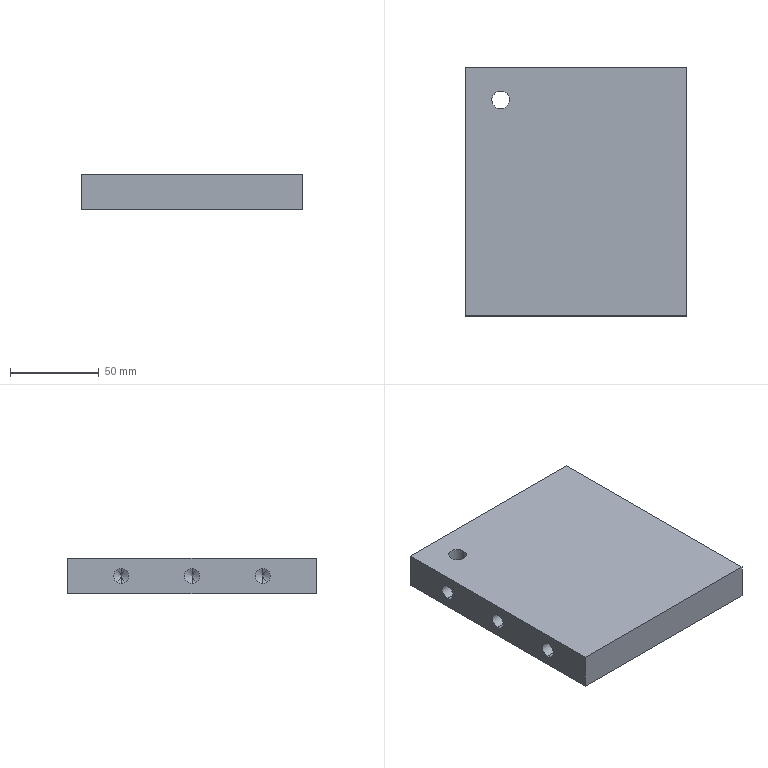Part | SolidWorks | features HoleWzd 2, Extrusion 1, ICE 1 | 1 solid | 32 faces | box 125 x 140 x 20 mm | volume 339828 mm3 | cylinder 14 | cone 12 | plane 6 | commonest cylinder face diameters 6.8 x6 8.5 x6 10 x2
STEP:
#1=CARTESIAN_POINT('',(-47.5,52.,0.));
#2=VERTEX_POINT('',#1);
#3=CARTESIAN_POINT('',(-37.5,52.,0.));
#4=VERTEX_POINT('',#3);
#5=CARTESIAN_POINT('',(-42.5,52.,0.));
#6=DIRECTION('',(0.,0.,1.));
#7=DIRECTION('',(1.,0.,0.));
#8=AXIS2_PLACEMENT_3D('',#5,#6,#7);
#9=CIRCLE('',#8,5.);
#10=EDGE_CURVE('',#2,#4,#9,.T.);
#11=ORIENTED_EDGE('',*,*,#10,.F.);
#12=CARTESIAN_POINT('',(-47.5,52.,20.));
#13=VERTEX_POINT('',#12);
#14=CARTESIAN_POINT('',(-47.5,52.,0.));
#15=DIRECTION('',(0.,0.,1.));
#16=VECTOR('',#15,1000.);
#17=LINE('',#14,#16);
#18=EDGE_CURVE('',#2,#13,#17,.T.);
#19=ORIENTED_EDGE('',*,*,#18,.T.);
#20=CARTESIAN_POINT('',(-37.5,52.,20.));
#21=VERTEX_POINT('',#20);
#22=CARTESIAN_POINT('',(-42.5,52.,20.));
#23=DIRECTION('',(0.,0.,1.));
#24=DIRECTION('',(1.,0.,0.));
#25=AXIS2_PLACEMENT_3D('',#22,#23,#24);
#26=CIRCLE('',#25,5.);
#27=EDGE_CURVE('',#13,#21,#26,.T.);
#28=ORIENTED_EDGE('',*,*,#27,.T.);
#29=CARTESIAN_POINT('',(-37.5,52.,0.));
#30=DIRECTION('',(0.,0.,1.));
#31=VECTOR('',#30,1000.);
#32=LINE('',#29,#31);
#33=EDGE_CURVE('',#4,#21,#32,.T.);
#34=ORIENTED_EDGE('',*,*,#33,.F.);
#35=EDGE_LOOP('',(#11,#19,#28,#34));
#36=FACE_OUTER_BOUND('',#35,.T.);
#37=CARTESIAN_POINT('',(-42.5,52.,0.));
#38=DIRECTION('',(0.,0.,1.));
#39=DIRECTION('',(1.,0.,0.));
#40=AXIS2_PLACEMENT_3D('',#37,#38,#39);
#41=CYLINDRICAL_SURFACE('',#40,5.);
#42=ADVANCED_FACE('',(#36),#41,.F.);
#43=CARTESIAN_POINT('',(40.25,58.,13.4));
#44=VERTEX_POINT('',#43);
#45=CARTESIAN_POINT('',(40.25,58.,6.6));
#46=VERTEX_POINT('',#45);
#47=CARTESIAN_POINT('',(40.25,58.,10.));
#48=DIRECTION('',(1.,0.,0.));
#49=DIRECTION('',(0.,0.,-1.));
#50=AXIS2_PLACEMENT_3D('',#47,#48,#49);
#51=CIRCLE('',#50,3.4);
#52=EDGE_CURVE('',#44,#46,#51,.T.);
#53=ORIENTED_EDGE('',*,*,#52,.F.);
#54=CARTESIAN_POINT('',(62.5,58.,13.4));
#55=VERTEX_POINT('',#54);
#56=CARTESIAN_POINT('',(62.5,58.,13.4));
#57=DIRECTION('',(1.,0.,0.));
#58=VECTOR('',#57,1000.);
#59=LINE('',#56,#58);
#60=EDGE_CURVE('',#44,#55,#59,.T.);
#61=ORIENTED_EDGE('',*,*,#60,.T.);
#62=CARTESIAN_POINT('',(62.5,58.,6.6));
#63=VERTEX_POINT('',#62);
#64=CARTESIAN_POINT('',(62.5,58.,10.));
#65=DIRECTION('',(1.,0.,0.));
#66=DIRECTION('',(0.,0.,-1.));
#67=AXIS2_PLACEMENT_3D('',#64,#65,#66);
#68=CIRCLE('',#67,3.4);
#69=EDGE_CURVE('',#55,#63,#68,.T.);
#70=ORIENTED_EDGE('',*,*,#69,.T.);
#71=CARTESIAN_POINT('',(62.5,58.,6.6));
#72=DIRECTION('',(1.,0.,0.));
#73=VECTOR('',#72,1000.);
#74=LINE('',#71,#73);
#75=EDGE_CURVE('',#46,#63,#74,.T.);
#76=ORIENTED_EDGE('',*,*,#75,.F.);
#77=EDGE_LOOP('',(#53,#61,#70,#76));
#78=FACE_OUTER_BOUND('',#77,.T.);
#79=CARTESIAN_POINT('',(62.5,58.,10.));
#80=DIRECTION('',(1.,0.,0.));
#81=DIRECTION('',(0.,0.,-1.));
#82=AXIS2_PLACEMENT_3D('',#79,#80,#81);
#83=CYLINDRICAL_SURFACE('',#82,3.4);
#84=ADVANCED_FACE('',(#78),#83,.F.);
#85=CARTESIAN_POINT('',(38.207,58.,10.));
#86=VERTEX_POINT('',#85);
#87=CARTESIAN_POINT('',(40.25,58.,6.6));
#88=DIRECTION('',(0.515,0.,-0.8572));
#89=VECTOR('',#88,1000.);
#90=LINE('',#87,#89);
#91=EDGE_CURVE('',#86,#46,#90,.T.);
#92=ORIENTED_EDGE('',*,*,#91,.F.);
#93=CARTESIAN_POINT('',(40.25,58.,13.4));
#94=DIRECTION('',(0.515,0.,0.8572));
#95=VECTOR('',#94,1000.);
#96=LINE('',#93,#95);
#97=EDGE_CURVE('',#86,#44,#96,.T.);
#98=ORIENTED_EDGE('',*,*,#97,.T.);
#99=ORIENTED_EDGE('',*,*,#52,.T.);
#100=EDGE_LOOP('',(#92,#98,#99));
#101=FACE_OUTER_BOUND('',#100,.T.);
#102=CARTESIAN_POINT('',(40.25,58.,10.));
#103=DIRECTION('',(1.,0.,0.));
#104=DIRECTION('',(0.,0.,-1.));
#105=AXIS2_PLACEMENT_3D('',#102,#103,#104);
#106=CONICAL_SURFACE('',#105,3.4,1.03);
#107=ADVANCED_FACE('',(#101),#106,.F.);
#108=CARTESIAN_POINT('',(40.25,0.,13.4));
#109=VERTEX_POINT('',#108);
#110=CARTESIAN_POINT('',(40.25,0.,6.6));
#111=VERTEX_POINT('',#110);
#112=CARTESIAN_POINT('',(40.25,0.,10.));
#113=DIRECTION('',(1.,0.,0.));
#114=DIRECTION('',(0.,0.,-1.));
#115=AXIS2_PLACEMENT_3D('',#112,#113,#114);
#116=CIRCLE('',#115,3.4);
#117=EDGE_CURVE('',#109,#111,#116,.T.);
#118=ORIENTED_EDGE('',*,*,#117,.F.);
#119=CARTESIAN_POINT('',(62.5,0.,13.4));
#120=VERTEX_POINT('',#119);
#121=CARTESIAN_POINT('',(62.5,0.,13.4));
#122=DIRECTION('',(1.,0.,0.));
#123=VECTOR('',#122,1000.);
#124=LINE('',#121,#123);
#125=EDGE_CURVE('',#109,#120,#124,.T.);
#126=ORIENTED_EDGE('',*,*,#125,.T.);
#127=CARTESIAN_POINT('',(62.5,0.,6.6));
#128=VERTEX_POINT('',#127);
#129=CARTESIAN_POINT('',(62.5,0.,10.));
#130=DIRECTION('',(1.,0.,0.));
#131=DIRECTION('',(0.,0.,-1.));
#132=AXIS2_PLACEMENT_3D('',#129,#130,#131);
#133=CIRCLE('',#132,3.4);
#134=EDGE_CURVE('',#120,#128,#133,.T.);
#135=ORIENTED_EDGE('',*,*,#134,.T.);
#136=CARTESIAN_POINT('',(62.5,0.,6.6));
#137=DIRECTION('',(1.,0.,0.));
#138=VECTOR('',#137,1000.);
#139=LINE('',#136,#138);
#140=EDGE_CURVE('',#111,#128,#139,.T.);
#141=ORIENTED_EDGE('',*,*,#140,.F.);
#142=EDGE_LOOP('',(#118,#126,#135,#141));
#143=FACE_OUTER_BOUND('',#142,.T.);
#144=CARTESIAN_POINT('',(62.5,0.,10.));
#145=DIRECTION('',(1.,0.,0.));
#146=DIRECTION('',(0.,0.,-1.));
#147=AXIS2_PLACEMENT_3D('',#144,#145,#146);
#148=CYLINDRICAL_SURFACE('',#147,3.4);
#149=ADVANCED_FACE('',(#143),#148,.F.);
#150=CARTESIAN_POINT('',(38.207,0.,10.));
#151=VERTEX_POINT('',#150);
#152=CARTESIAN_POINT('',(40.25,0.,6.6));
#153=DIRECTION('',(0.515,0.,-0.8572));
#154=VECTOR('',#153,1000.);
#155=LINE('',#152,#154);
#156=EDGE_CURVE('',#151,#111,#155,.T.);
#157=ORIENTED_EDGE('',*,*,#156,.F.);
#158=CARTESIAN_POINT('',(40.25,0.,13.4));
#159=DIRECTION('',(0.515,0.,0.8572));
#160=VECTOR('',#159,1000.);
#161=LINE('',#158,#160);
#162=EDGE_CURVE('',#151,#109,#161,.T.);
#163=ORIENTED_EDGE('',*,*,#162,.T.);
#164=ORIENTED_EDGE('',*,*,#117,.T.);
#165=EDGE_LOOP('',(#157,#163,#164));
#166=FACE_OUTER_BOUND('',#165,.T.);
#167=CARTESIAN_POINT('',(40.25,0.,10.));
#168=DIRECTION('',(1.,0.,0.));
#169=DIRECTION('',(0.,0.,-1.));
#170=AXIS2_PLACEMENT_3D('',#167,#168,#169);
#171=CONICAL_SURFACE('',#170,3.4,1.03);
#172=ADVANCED_FACE('',(#166),#171,.F.);
#173=CARTESIAN_POINT('',(40.25,-58.,13.4));
#174=VERTEX_POINT('',#173);
#175=CARTESIAN_POINT('',(40.25,-58.,6.6));
#176=VERTEX_POINT('',#175);
#177=CARTESIAN_POINT('',(40.25,-58.,10.));
#178=DIRECTION('',(1.,0.,0.));
#179=DIRECTION('',(0.,0.,-1.));
#180=AXIS2_PLACEMENT_3D('',#177,#178,#179);
#181=CIRCLE('',#180,3.4);
#182=EDGE_CURVE('',#174,#176,#181,.T.);
#183=ORIENTED_EDGE('',*,*,#182,.F.);
#184=CARTESIAN_POINT('',(62.5,-58.,13.4));
#185=VERTEX_POINT('',#184);
#186=CARTESIAN_POINT('',(62.5,-58.,13.4));
#187=DIRECTION('',(1.,0.,0.));
#188=VECTOR('',#187,1000.);
#189=LINE('',#186,#188);
#190=EDGE_CURVE('',#174,#185,#189,.T.);
#191=ORIENTED_EDGE('',*,*,#190,.T.);
#192=CARTESIAN_POINT('',(62.5,-58.,6.6));
#193=VERTEX_POINT('',#192);
#194=CARTESIAN_POINT('',(62.5,-58.,10.));
#195=DIRECTION('',(1.,0.,0.));
#196=DIRECTION('',(0.,0.,-1.));
#197=AXIS2_PLACEMENT_3D('',#194,#195,#196);
#198=CIRCLE('',#197,3.4);
#199=EDGE_CURVE('',#185,#193,#198,.T.);
#200=ORIENTED_EDGE('',*,*,#199,.T.);
#201=CARTESIAN_POINT('',(62.5,-58.,6.6));
#202=DIRECTION('',(1.,0.,0.));
#203=VECTOR('',#202,1000.);
#204=LINE('',#201,#203);
#205=EDGE_CURVE('',#176,#193,#204,.T.);
#206=ORIENTED_EDGE('',*,*,#205,.F.);
#207=EDGE_LOOP('',(#183,#191,#200,#206));
#208=FACE_OUTER_BOUND('',#207,.T.);
#209=CARTESIAN_POINT('',(62.5,-58.,10.));
#210=DIRECTION('',(1.,0.,0.));
#211=DIRECTION('',(0.,0.,-1.));
#212=AXIS2_PLACEMENT_3D('',#209,#210,#211);
#213=CYLINDRICAL_SURFACE('',#212,3.4);
#214=ADVANCED_FACE('',(#208),#213,.F.);
#215=CARTESIAN_POINT('',(38.207,-58.,10.));
#216=VERTEX_POINT('',#215);
#217=CARTESIAN_POINT('',(40.25,-58.,6.6));
#218=DIRECTION('',(0.515,0.,-0.8572));
#219=VECTOR('',#218,1000.);
#220=LINE('',#217,#219);
#221=EDGE_CURVE('',#216,#176,#220,.T.);
#222=ORIENTED_EDGE('',*,*,#221,.F.);
#223=CARTESIAN_POINT('',(40.25,-58.,13.4));
#224=DIRECTION('',(0.515,0.,0.8572));
#225=VECTOR('',#224,1000.);
#226=LINE('',#223,#225);
#227=EDGE_CURVE('',#216,#174,#226,.T.);
#228=ORIENTED_EDGE('',*,*,#227,.T.);
#229=ORIENTED_EDGE('',*,*,#182,.T.);
#230=EDGE_LOOP('',(#222,#228,#229));
#231=FACE_OUTER_BOUND('',#230,.T.);
#232=CARTESIAN_POINT('',(40.25,-58.,10.));
#233=DIRECTION('',(1.,0.,0.));
#234=DIRECTION('',(0.,0.,-1.));
#235=AXIS2_PLACEMENT_3D('',#232,#233,#234);
#236=CONICAL_SURFACE('',#235,3.4,1.03);
#237=ADVANCED_FACE('',(#231),#236,.F.);
#238=CARTESIAN_POINT('',(-27.5,40.,5.75));
#239=VERTEX_POINT('',#238);
#240=CARTESIAN_POINT('',(-27.5,40.,14.25));
#241=VERTEX_POINT('',#240);
#242=CARTESIAN_POINT('',(-27.5,40.,10.));
#243=DIRECTION('',(-1.,0.,0.));
#244=DIRECTION('',(0.,0.,1.));
#245=AXIS2_PLACEMENT_3D('',#242,#243,#244);
#246=CIRCLE('',#245,4.25);
#247=EDGE_CURVE('',#239,#241,#246,.T.);
#248=ORIENTED_EDGE('',*,*,#247,.F.);
#249=CARTESIAN_POINT('',(-62.5,40.,5.75));
#250=VERTEX_POINT('',#249);
#251=CARTESIAN_POINT('',(-62.5,40.,5.75));
#252=DIRECTION('',(-1.,0.,0.));
#253=VECTOR('',#252,1000.);
#254=LINE('',#251,#253);
#255=EDGE_CURVE('',#239,#250,#254,.T.);
#256=ORIENTED_EDGE('',*,*,#255,.T.);
#257=CARTESIAN_POINT('',(-62.5,40.,14.25));
#258=VERTEX_POINT('',#257);
#259=CARTESIAN_POINT('',(-62.5,40.,10.));
#260=DIRECTION('',(-1.,0.,0.));
#261=DIRECTION('',(0.,0.,1.));
#262=AXIS2_PLACEMENT_3D('',#259,#260,#261);
#263=CIRCLE('',#262,4.25);
#264=EDGE_CURVE('',#250,#258,#263,.T.);
#265=ORIENTED_EDGE('',*,*,#264,.T.);
#266=CARTESIAN_POINT('',(-62.5,40.,14.25));
#267=DIRECTION('',(-1.,0.,0.));
#268=VECTOR('',#267,1000.);
#269=LINE('',#266,#268);
#270=EDGE_CURVE('',#241,#258,#269,.T.);
#271=ORIENTED_EDGE('',*,*,#270,.F.);
#272=EDGE_LOOP('',(#248,#256,#265,#271));
#273=FACE_OUTER_BOUND('',#272,.T.);
#274=CARTESIAN_POINT('',(-62.5,40.,10.));
#275=DIRECTION('',(-1.,0.,0.));
#276=DIRECTION('',(0.,0.,1.));
#277=AXIS2_PLACEMENT_3D('',#274,#275,#276);
#278=CYLINDRICAL_SURFACE('',#277,4.25);
#279=ADVANCED_FACE('',(#273),#278,.F.);
#280=CARTESIAN_POINT('',(-24.946,40.,10.));
#281=VERTEX_POINT('',#280);
#282=CARTESIAN_POINT('',(-27.5,40.,14.25));
#283=DIRECTION('',(-0.515,0.,0.8572));
#284=VECTOR('',#283,1000.);
#285=LINE('',#282,#284);
#286=EDGE_CURVE('',#281,#241,#285,.T.);
#287=ORIENTED_EDGE('',*,*,#286,.F.);
#288=CARTESIAN_POINT('',(-27.5,40.,5.75));
#289=DIRECTION('',(-0.515,0.,-0.8572));
#290=VECTOR('',#289,1000.);
#291=LINE('',#288,#290);
#292=EDGE_CURVE('',#281,#239,#291,.T.);
#293=ORIENTED_EDGE('',*,*,#292,.T.);
#294=ORIENTED_EDGE('',*,*,#247,.T.);
#295=EDGE_LOOP('',(#287,#293,#294));
#296=FACE_OUTER_BOUND('',#295,.T.);
#297=CARTESIAN_POINT('',(-27.5,40.,10.));
#298=DIRECTION('',(-1.,0.,0.));
#299=DIRECTION('',(0.,0.,1.));
#300=AXIS2_PLACEMENT_3D('',#297,#298,#299);
#301=CONICAL_SURFACE('',#300,4.25,1.03);
#302=ADVANCED_FACE('',(#296),#301,.F.);
#303=CARTESIAN_POINT('',(-27.5,0.,5.75));
#304=VERTEX_POINT('',#303);
#305=CARTESIAN_POINT('',(-27.5,0.,14.25));
#306=VERTEX_POINT('',#305);
#307=CARTESIAN_POINT('',(-27.5,0.,10.));
#308=DIRECTION('',(-1.,0.,0.));
#309=DIRECTION('',(0.,0.,1.));
#310=AXIS2_PLACEMENT_3D('',#307,#308,#309);
#311=CIRCLE('',#310,4.25);
#312=EDGE_CURVE('',#304,#306,#311,.T.);
#313=ORIENTED_EDGE('',*,*,#312,.F.);
#314=CARTESIAN_POINT('',(-62.5,0.,5.75));
#315=VERTEX_POINT('',#314);
#316=CARTESIAN_POINT('',(-62.5,0.,5.75));
#317=DIRECTION('',(-1.,0.,0.));
#318=VECTOR('',#317,1000.);
#319=LINE('',#316,#318);
#320=EDGE_CURVE('',#304,#315,#319,.T.);
#321=ORIENTED_EDGE('',*,*,#320,.T.);
#322=CARTESIAN_POINT('',(-62.5,0.,14.25));
#323=VERTEX_POINT('',#322);
#324=CARTESIAN_POINT('',(-62.5,0.,10.));
#325=DIRECTION('',(-1.,0.,0.));
#326=DIRECTION('',(0.,0.,1.));
#327=AXIS2_PLACEMENT_3D('',#324,#325,#326);
#328=CIRCLE('',#327,4.25);
#329=EDGE_CURVE('',#315,#323,#328,.T.);
#330=ORIENTED_EDGE('',*,*,#329,.T.);
#331=CARTESIAN_POINT('',(-62.5,0.,14.25));
#332=DIRECTION('',(-1.,0.,0.));
#333=VECTOR('',#332,1000.);
#334=LINE('',#331,#333);
#335=EDGE_CURVE('',#306,#323,#334,.T.);
#336=ORIENTED_EDGE('',*,*,#335,.F.);
#337=EDGE_LOOP('',(#313,#321,#330,#336));
#338=FACE_OUTER_BOUND('',#337,.T.);
#339=CARTESIAN_POINT('',(-62.5,0.,10.));
#340=DIRECTION('',(-1.,0.,0.));
#341=DIRECTION('',(0.,0.,1.));
#342=AXIS2_PLACEMENT_3D('',#339,#340,#341);
#343=CYLINDRICAL_SURFACE('',#342,4.25);
#344=ADVANCED_FACE('',(#338),#343,.F.);
#345=CARTESIAN_POINT('',(-24.946,0.,10.));
#346=VERTEX_POINT('',#345);
#347=CARTESIAN_POINT('',(-27.5,0.,14.25));
#348=DIRECTION('',(-0.515,0.,0.8572));
#349=VECTOR('',#348,1000.);
#350=LINE('',#347,#349);
#351=EDGE_CURVE('',#346,#306,#350,.T.);
#352=ORIENTED_EDGE('',*,*,#351,.F.);
#353=CARTESIAN_POINT('',(-27.5,0.,5.75));
#354=DIRECTION('',(-0.515,0.,-0.8572));
#355=VECTOR('',#354,1000.);
#356=LINE('',#353,#355);
#357=EDGE_CURVE('',#346,#304,#356,.T.);
#358=ORIENTED_EDGE('',*,*,#357,.T.);
#359=ORIENTED_EDGE('',*,*,#312,.T.);
#360=EDGE_LOOP('',(#352,#358,#359));
#361=FACE_OUTER_BOUND('',#360,.T.);
#362=CARTESIAN_POINT('',(-27.5,0.,10.));
#363=DIRECTION('',(-1.,0.,0.));
#364=DIRECTION('',(0.,0.,1.));
#365=AXIS2_PLACEMENT_3D('',#362,#363,#364);
#366=CONICAL_SURFACE('',#365,4.25,1.03);
#367=ADVANCED_FACE('',(#361),#366,.F.);
#368=CARTESIAN_POINT('',(-27.5,-40.,5.75));
#369=VERTEX_POINT('',#368);
#370=CARTESIAN_POINT('',(-27.5,-40.,14.25));
#371=VERTEX_POINT('',#370);
#372=CARTESIAN_POINT('',(-27.5,-40.,10.));
#373=DIRECTION('',(-1.,0.,0.));
#374=DIRECTION('',(0.,0.,1.));
#375=AXIS2_PLACEMENT_3D('',#372,#373,#374);
#376=CIRCLE('',#375,4.25);
#377=EDGE_CURVE('',#369,#371,#376,.T.);
#378=ORIENTED_EDGE('',*,*,#377,.F.);
#379=CARTESIAN_POINT('',(-62.5,-40.,5.75));
#380=VERTEX_POINT('',#379);
#381=CARTESIAN_POINT('',(-62.5,-40.,5.75));
#382=DIRECTION('',(-1.,0.,0.));
#383=VECTOR('',#382,1000.);
#384=LINE('',#381,#383);
#385=EDGE_CURVE('',#369,#380,#384,.T.);
#386=ORIENTED_EDGE('',*,*,#385,.T.);
#387=CARTESIAN_POINT('',(-62.5,-40.,14.25));
#388=VERTEX_POINT('',#387);
#389=CARTESIAN_POINT('',(-62.5,-40.,10.));
#390=DIRECTION('',(-1.,0.,0.));
#391=DIRECTION('',(0.,0.,1.));
#392=AXIS2_PLACEMENT_3D('',#389,#390,#391);
#393=CIRCLE('',#392,4.25);
#394=EDGE_CURVE('',#380,#388,#393,.T.);
#395=ORIENTED_EDGE('',*,*,#394,.T.);
#396=CARTESIAN_POINT('',(-62.5,-40.,14.25));
#397=DIRECTION('',(-1.,0.,0.));
#398=VECTOR('',#397,1000.);
#399=LINE('',#396,#398);
#400=EDGE_CURVE('',#371,#388,#399,.T.);
#401=ORIENTED_EDGE('',*,*,#400,.F.);
#402=EDGE_LOOP('',(#378,#386,#395,#401));
#403=FACE_OUTER_BOUND('',#402,.T.);
#404=CARTESIAN_POINT('',(-62.5,-40.,10.));
#405=DIRECTION('',(-1.,0.,0.));
#406=DIRECTION('',(0.,0.,1.));
#407=AXIS2_PLACEMENT_3D('',#404,#405,#406);
#408=CYLINDRICAL_SURFACE('',#407,4.25);
#409=ADVANCED_FACE('',(#403),#408,.F.);
#410=CARTESIAN_POINT('',(-24.946,-40.,10.));
#411=VERTEX_POINT('',#410);
#412=CARTESIAN_POINT('',(-27.5,-40.,14.25));
#413=DIRECTION('',(-0.515,0.,0.8572));
#414=VECTOR('',#413,1000.);
#415=LINE('',#412,#414);
#416=EDGE_CURVE('',#411,#371,#415,.T.);
#417=ORIENTED_EDGE('',*,*,#416,.F.);
#418=CARTESIAN_POINT('',(-27.5,-40.,5.75));
#419=DIRECTION('',(-0.515,0.,-0.8572));
#420=VECTOR('',#419,1000.);
#421=LINE('',#418,#420);
#422=EDGE_CURVE('',#411,#369,#421,.T.);
#423=ORIENTED_EDGE('',*,*,#422,.T.);
#424=ORIENTED_EDGE('',*,*,#377,.T.);
#425=EDGE_LOOP('',(#417,#423,#424));
#426=FACE_OUTER_BOUND('',#425,.T.);
#427=CARTESIAN_POINT('',(-27.5,-40.,10.));
#428=DIRECTION('',(-1.,0.,0.));
#429=DIRECTION('',(0.,0.,1.));
#430=AXIS2_PLACEMENT_3D('',#427,#428,#429);
#431=CONICAL_SURFACE('',#430,4.25,1.03);
#432=ADVANCED_FACE('',(#426),#431,.F.);
#433=CARTESIAN_POINT('',(62.5,58.,10.));
#434=DIRECTION('',(1.,0.,0.));
#435=DIRECTION('',(0.,0.,-1.));
#436=AXIS2_PLACEMENT_3D('',#433,#434,#435);
#437=CIRCLE('',#436,3.4);
#438=EDGE_CURVE('',#63,#55,#437,.T.);
#439=ORIENTED_EDGE('',*,*,#438,.F.);
#440=ORIENTED_EDGE('',*,*,#69,.F.);
#441=EDGE_LOOP('',(#439,#440));
#442=FACE_BOUND('',#441,.T.);
#443=CARTESIAN_POINT('',(62.5,0.,10.));
#444=DIRECTION('',(1.,0.,0.));
#445=DIRECTION('',(0.,0.,-1.));
#446=AXIS2_PLACEMENT_3D('',#443,#444,#445);
#447=CIRCLE('',#446,3.4);
#448=EDGE_CURVE('',#128,#120,#447,.T.);
#449=ORIENTED_EDGE('',*,*,#448,.F.);
#450=ORIENTED_EDGE('',*,*,#134,.F.);
#451=EDGE_LOOP('',(#449,#450));
#452=FACE_BOUND('',#451,.T.);
#453=CARTESIAN_POINT('',(62.5,-58.,10.));
#454=DIRECTION('',(1.,0.,0.));
#455=DIRECTION('',(0.,0.,-1.));
#456=AXIS2_PLACEMENT_3D('',#453,#454,#455);
#457=CIRCLE('',#456,3.4);
#458=EDGE_CURVE('',#193,#185,#457,.T.);
#459=ORIENTED_EDGE('',*,*,#458,.F.);
#460=ORIENTED_EDGE('',*,*,#199,.F.);
#461=EDGE_LOOP('',(#459,#460));
#462=FACE_BOUND('',#461,.T.);
#463=CARTESIAN_POINT('',(62.5,-70.,0.));
#464=VERTEX_POINT('',#463);
#465=CARTESIAN_POINT('',(62.5,70.,0.));
#466=VERTEX_POINT('',#465);
#467=CARTESIAN_POINT('',(62.5,70.,0.));
#468=DIRECTION('',(0.,1.,0.));
#469=VECTOR('',#468,1000.);
#470=LINE('',#467,#469);
#471=EDGE_CURVE('',#464,#466,#470,.T.);
#472=ORIENTED_EDGE('',*,*,#471,.T.);
#473=CARTESIAN_POINT('',(62.5,70.,20.));
#474=VERTEX_POINT('',#473);
#475=CARTESIAN_POINT('',(62.5,70.,20.));
#476=DIRECTION('',(0.,0.,-1.));
#477=VECTOR('',#476,1000.);
#478=LINE('',#475,#477);
#479=EDGE_CURVE('',#474,#466,#478,.T.);
#480=ORIENTED_EDGE('',*,*,#479,.F.);
#481=CARTESIAN_POINT('',(62.5,-70.,20.));
#482=VERTEX_POINT('',#481);
#483=CARTESIAN_POINT('',(62.5,70.,20.));
#484=DIRECTION('',(0.,1.,0.));
#485=VECTOR('',#484,1000.);
#486=LINE('',#483,#485);
#487=EDGE_CURVE('',#482,#474,#486,.T.);
#488=ORIENTED_EDGE('',*,*,#487,.F.);
#489=CARTESIAN_POINT('',(62.5,-70.,20.));
#490=DIRECTION('',(0.,0.,-1.));
#491=VECTOR('',#490,1000.);
#492=LINE('',#489,#491);
#493=EDGE_CURVE('',#482,#464,#492,.T.);
#494=ORIENTED_EDGE('',*,*,#493,.T.);
#495=EDGE_LOOP('',(#472,#480,#488,#494));
#496=FACE_OUTER_BOUND('',#495,.T.);
#497=CARTESIAN_POINT('',(62.5,70.,20.));
#498=DIRECTION('',(-1.,0.,0.));
#499=DIRECTION('',(0.,-1.,0.));
#500=AXIS2_PLACEMENT_3D('',#497,#498,#499);
#501=PLANE('',#500);
#502=ADVANCED_FACE('',(#442,#452,#462,#496),#501,.F.);
#503=CARTESIAN_POINT('',(-62.5,70.,0.));
#504=VERTEX_POINT('',#503);
#505=CARTESIAN_POINT('',(-62.5,70.,0.));
#506=DIRECTION('',(-1.,0.,0.));
#507=VECTOR('',#506,1000.);
#508=LINE('',#505,#507);
#509=EDGE_CURVE('',#466,#504,#508,.T.);
#510=ORIENTED_EDGE('',*,*,#509,.T.);
#511=CARTESIAN_POINT('',(-62.5,70.,20.));
#512=VERTEX_POINT('',#511);
#513=CARTESIAN_POINT('',(-62.5,70.,20.));
#514=DIRECTION('',(0.,0.,-1.));
#515=VECTOR('',#514,1000.);
#516=LINE('',#513,#515);
#517=EDGE_CURVE('',#512,#504,#516,.T.);
#518=ORIENTED_EDGE('',*,*,#517,.F.);
#519=CARTESIAN_POINT('',(-62.5,70.,20.));
#520=DIRECTION('',(-1.,0.,0.));
#521=VECTOR('',#520,1000.);
#522=LINE('',#519,#521);
#523=EDGE_CURVE('',#474,#512,#522,.T.);
#524=ORIENTED_EDGE('',*,*,#523,.F.);
#525=ORIENTED_EDGE('',*,*,#479,.T.);
#526=EDGE_LOOP('',(#510,#518,#524,#525));
#527=FACE_OUTER_BOUND('',#526,.T.);
#528=CARTESIAN_POINT('',(-62.5,70.,20.));
#529=DIRECTION('',(0.,-1.,0.));
#530=DIRECTION('',(0.,0.,-1.));
#531=AXIS2_PLACEMENT_3D('',#528,#529,#530);
#532=PLANE('',#531);
#533=ADVANCED_FACE('',(#527),#532,.F.);
#534=CARTESIAN_POINT('',(-62.5,40.,10.));
#535=DIRECTION('',(-1.,0.,0.));
#536=DIRECTION('',(0.,0.,1.));
#537=AXIS2_PLACEMENT_3D('',#534,#535,#536);
#538=CIRCLE('',#537,4.25);
#539=EDGE_CURVE('',#258,#250,#538,.T.);
#540=ORIENTED_EDGE('',*,*,#539,.F.);
#541=ORIENTED_EDGE('',*,*,#264,.F.);
#542=EDGE_LOOP('',(#540,#541));
#543=FACE_BOUND('',#542,.T.);
#544=CARTESIAN_POINT('',(-62.5,0.,10.));
#545=DIRECTION('',(-1.,0.,0.));
#546=DIRECTION('',(0.,0.,1.));
#547=AXIS2_PLACEMENT_3D('',#544,#545,#546);
#548=CIRCLE('',#547,4.25);
#549=EDGE_CURVE('',#323,#315,#548,.T.);
#550=ORIENTED_EDGE('',*,*,#549,.F.);
#551=ORIENTED_EDGE('',*,*,#329,.F.);
#552=EDGE_LOOP('',(#550,#551));
#553=FACE_BOUND('',#552,.T.);
#554=CARTESIAN_POINT('',(-62.5,-40.,10.));
#555=DIRECTION('',(-1.,0.,0.));
#556=DIRECTION('',(0.,0.,1.));
#557=AXIS2_PLACEMENT_3D('',#554,#555,#556);
#558=CIRCLE('',#557,4.25);
#559=EDGE_CURVE('',#388,#380,#558,.T.);
#560=ORIENTED_EDGE('',*,*,#559,.F.);
#561=ORIENTED_EDGE('',*,*,#394,.F.);
#562=EDGE_LOOP('',(#560,#561));
#563=FACE_BOUND('',#562,.T.);
#564=CARTESIAN_POINT('',(-62.5,-70.,0.));
#565=VERTEX_POINT('',#564);
#566=CARTESIAN_POINT('',(-62.5,70.,0.));
#567=DIRECTION('',(0.,-1.,0.));
#568=VECTOR('',#567,1000.);
#569=LINE('',#566,#568);
#570=EDGE_CURVE('',#504,#565,#569,.T.);
#571=ORIENTED_EDGE('',*,*,#570,.T.);
#572=CARTESIAN_POINT('',(-62.5,-70.,20.));
#573=VERTEX_POINT('',#572);
#574=CARTESIAN_POINT('',(-62.5,-70.,20.));
#575=DIRECTION('',(0.,0.,-1.));
#576=VECTOR('',#575,1000.);
#577=LINE('',#574,#576);
#578=EDGE_CURVE('',#573,#565,#577,.T.);
#579=ORIENTED_EDGE('',*,*,#578,.F.);
#580=CARTESIAN_POINT('',(-62.5,70.,20.));
#581=DIRECTION('',(0.,-1.,0.));
#582=VECTOR('',#581,1000.);
#583=LINE('',#580,#582);
#584=EDGE_CURVE('',#512,#573,#583,.T.);
#585=ORIENTED_EDGE('',*,*,#584,.F.);
#586=ORIENTED_EDGE('',*,*,#517,.T.);
#587=EDGE_LOOP('',(#571,#579,#585,#586));
#588=FACE_OUTER_BOUND('',#587,.T.);
#589=CARTESIAN_POINT('',(-62.5,70.,20.));
#590=DIRECTION('',(1.,0.,0.));
#591=DIRECTION('',(0.,1.,0.));
#592=AXIS2_PLACEMENT_3D('',#589,#590,#591);
#593=PLANE('',#592);
#594=ADVANCED_FACE('',(#543,#553,#563,#588),#593,.F.);
#595=CARTESIAN_POINT('',(-62.5,-70.,0.));
#596=DIRECTION('',(1.,0.,0.));
#597=VECTOR('',#596,1000.);
#598=LINE('',#595,#597);
#599=EDGE_CURVE('',#565,#464,#598,.T.);
#600=ORIENTED_EDGE('',*,*,#599,.T.);
#601=ORIENTED_EDGE('',*,*,#493,.F.);
#602=CARTESIAN_POINT('',(-62.5,-70.,20.));
#603=DIRECTION('',(1.,0.,0.));
#604=VECTOR('',#603,1000.);
#605=LINE('',#602,#604);
#606=EDGE_CURVE('',#573,#482,#605,.T.);
#607=ORIENTED_EDGE('',*,*,#606,.F.);
#608=ORIENTED_EDGE('',*,*,#578,.T.);
#609=EDGE_LOOP('',(#600,#601,#607,#608));
#610=FACE_OUTER_BOUND('',#609,.T.);
#611=CARTESIAN_POINT('',(-62.5,-70.,20.));
#612=DIRECTION('',(0.,1.,0.));
#613=DIRECTION('',(0.,0.,1.));
#614=AXIS2_PLACEMENT_3D('',#611,#612,#613);
#615=PLANE('',#614);
#616=ADVANCED_FACE('',(#610),#615,.F.);
#617=CARTESIAN_POINT('',(-42.5,52.,20.));
#618=DIRECTION('',(0.,0.,1.));
#619=DIRECTION('',(1.,0.,0.));
#620=AXIS2_PLACEMENT_3D('',#617,#618,#619);
#621=CIRCLE('',#620,5.);
#622=EDGE_CURVE('',#21,#13,#621,.T.);
#623=ORIENTED_EDGE('',*,*,#622,.F.);
#624=ORIENTED_EDGE('',*,*,#27,.F.);
#625=EDGE_LOOP('',(#623,#624));
#626=FACE_BOUND('',#625,.T.);
#627=ORIENTED_EDGE('',*,*,#487,.T.);
#628=ORIENTED_EDGE('',*,*,#523,.T.);
#629=ORIENTED_EDGE('',*,*,#584,.T.);
#630=ORIENTED_EDGE('',*,*,#606,.T.);
#631=EDGE_LOOP('',(#627,#628,#629,#630));
#632=FACE_OUTER_BOUND('',#631,.T.);
#633=CARTESIAN_POINT('',(0.,0.,20.));
#634=DIRECTION('',(0.,0.,1.));
#635=DIRECTION('',(1.,0.,0.));
#636=AXIS2_PLACEMENT_3D('',#633,#634,#635);
#637=PLANE('',#636);
#638=ADVANCED_FACE('',(#626,#632),#637,.T.);
#639=CARTESIAN_POINT('',(-42.5,52.,0.));
#640=DIRECTION('',(0.,0.,1.));
#641=DIRECTION('',(1.,0.,0.));
#642=AXIS2_PLACEMENT_3D('',#639,#640,#641);
#643=CIRCLE('',#642,5.);
#644=EDGE_CURVE('',#4,#2,#643,.T.);
#645=ORIENTED_EDGE('',*,*,#644,.T.);
#646=ORIENTED_EDGE('',*,*,#10,.T.);
#647=EDGE_LOOP('',(#645,#646));
#648=FACE_BOUND('',#647,.T.);
#649=ORIENTED_EDGE('',*,*,#471,.F.);
#650=ORIENTED_EDGE('',*,*,#599,.F.);
#651=ORIENTED_EDGE('',*,*,#570,.F.);
#652=ORIENTED_EDGE('',*,*,#509,.F.);
#653=EDGE_LOOP('',(#649,#650,#651,#652));
#654=FACE_OUTER_BOUND('',#653,.T.);
#655=CARTESIAN_POINT('',(0.,0.,0.));
#656=DIRECTION('',(0.,0.,1.));
#657=DIRECTION('',(1.,0.,0.));
#658=AXIS2_PLACEMENT_3D('',#655,#656,#657);
#659=PLANE('',#658);
#660=ADVANCED_FACE('',(#648,#654),#659,.F.);
#661=ORIENTED_EDGE('',*,*,#422,.F.);
#662=ORIENTED_EDGE('',*,*,#416,.T.);
#663=CARTESIAN_POINT('',(-27.5,-40.,10.));
#664=DIRECTION('',(-1.,0.,0.));
#665=DIRECTION('',(0.,0.,1.));
#666=AXIS2_PLACEMENT_3D('',#663,#664,#665);
#667=CIRCLE('',#666,4.25);
#668=EDGE_CURVE('',#371,#369,#667,.T.);
#669=ORIENTED_EDGE('',*,*,#668,.T.);
#670=EDGE_LOOP('',(#661,#662,#669));
#671=FACE_OUTER_BOUND('',#670,.T.);
#672=CARTESIAN_POINT('',(-27.5,-40.,10.));
#673=DIRECTION('',(-1.,0.,0.));
#674=DIRECTION('',(0.,0.,1.));
#675=AXIS2_PLACEMENT_3D('',#672,#673,#674);
#676=CONICAL_SURFACE('',#675,4.25,1.03);
#677=ADVANCED_FACE('',(#671),#676,.F.);
#678=ORIENTED_EDGE('',*,*,#385,.F.);
#679=ORIENTED_EDGE('',*,*,#668,.F.);
#680=ORIENTED_EDGE('',*,*,#400,.T.);
#681=ORIENTED_EDGE('',*,*,#559,.T.);
#682=EDGE_LOOP('',(#678,#679,#680,#681));
#683=FACE_OUTER_BOUND('',#682,.T.);
#684=CARTESIAN_POINT('',(-62.5,-40.,10.));
#685=DIRECTION('',(-1.,0.,0.));
#686=DIRECTION('',(0.,0.,1.));
#687=AXIS2_PLACEMENT_3D('',#684,#685,#686);
#688=CYLINDRICAL_SURFACE('',#687,4.25);
#689=ADVANCED_FACE('',(#683),#688,.F.);
#690=ORIENTED_EDGE('',*,*,#357,.F.);
#691=ORIENTED_EDGE('',*,*,#351,.T.);
#692=CARTESIAN_POINT('',(-27.5,0.,10.));
#693=DIRECTION('',(-1.,0.,0.));
#694=DIRECTION('',(0.,0.,1.));
#695=AXIS2_PLACEMENT_3D('',#692,#693,#694);
#696=CIRCLE('',#695,4.25);
#697=EDGE_CURVE('',#306,#304,#696,.T.);
#698=ORIENTED_EDGE('',*,*,#697,.T.);
#699=EDGE_LOOP('',(#690,#691,#698));
#700=FACE_OUTER_BOUND('',#699,.T.);
#701=CARTESIAN_POINT('',(-27.5,0.,10.));
#702=DIRECTION('',(-1.,0.,0.));
#703=DIRECTION('',(0.,0.,1.));
#704=AXIS2_PLACEMENT_3D('',#701,#702,#703);
#705=CONICAL_SURFACE('',#704,4.25,1.03);
#706=ADVANCED_FACE('',(#700),#705,.F.);
#707=ORIENTED_EDGE('',*,*,#320,.F.);
#708=ORIENTED_EDGE('',*,*,#697,.F.);
#709=ORIENTED_EDGE('',*,*,#335,.T.);
#710=ORIENTED_EDGE('',*,*,#549,.T.);
#711=EDGE_LOOP('',(#707,#708,#709,#710));
#712=FACE_OUTER_BOUND('',#711,.T.);
#713=CARTESIAN_POINT('',(-62.5,0.,10.));
#714=DIRECTION('',(-1.,0.,0.));
#715=DIRECTION('',(0.,0.,1.));
#716=AXIS2_PLACEMENT_3D('',#713,#714,#715);
#717=CYLINDRICAL_SURFACE('',#716,4.25);
#718=ADVANCED_FACE('',(#712),#717,.F.);
#719=ORIENTED_EDGE('',*,*,#292,.F.);
#720=ORIENTED_EDGE('',*,*,#286,.T.);
#721=CARTESIAN_POINT('',(-27.5,40.,10.));
#722=DIRECTION('',(-1.,0.,0.));
#723=DIRECTION('',(0.,0.,1.));
#724=AXIS2_PLACEMENT_3D('',#721,#722,#723);
#725=CIRCLE('',#724,4.25);
#726=EDGE_CURVE('',#241,#239,#725,.T.);
#727=ORIENTED_EDGE('',*,*,#726,.T.);
#728=EDGE_LOOP('',(#719,#720,#727));
#729=FACE_OUTER_BOUND('',#728,.T.);
#730=CARTESIAN_POINT('',(-27.5,40.,10.));
#731=DIRECTION('',(-1.,0.,0.));
#732=DIRECTION('',(0.,0.,1.));
#733=AXIS2_PLACEMENT_3D('',#730,#731,#732);
#734=CONICAL_SURFACE('',#733,4.25,1.03);
#735=ADVANCED_FACE('',(#729),#734,.F.);
#736=ORIENTED_EDGE('',*,*,#255,.F.);
#737=ORIENTED_EDGE('',*,*,#726,.F.);
#738=ORIENTED_EDGE('',*,*,#270,.T.);
#739=ORIENTED_EDGE('',*,*,#539,.T.);
#740=EDGE_LOOP('',(#736,#737,#738,#739));
#741=FACE_OUTER_BOUND('',#740,.T.);
#742=CARTESIAN_POINT('',(-62.5,40.,10.));
#743=DIRECTION('',(-1.,0.,0.));
#744=DIRECTION('',(0.,0.,1.));
#745=AXIS2_PLACEMENT_3D('',#742,#743,#744);
#746=CYLINDRICAL_SURFACE('',#745,4.25);
#747=ADVANCED_FACE('',(#741),#746,.F.);
#748=ORIENTED_EDGE('',*,*,#227,.F.);
#749=ORIENTED_EDGE('',*,*,#221,.T.);
#750=CARTESIAN_POINT('',(40.25,-58.,10.));
#751=DIRECTION('',(1.,0.,0.));
#752=DIRECTION('',(0.,0.,-1.));
#753=AXIS2_PLACEMENT_3D('',#750,#751,#752);
#754=CIRCLE('',#753,3.4);
#755=EDGE_CURVE('',#176,#174,#754,.T.);
#756=ORIENTED_EDGE('',*,*,#755,.T.);
#757=EDGE_LOOP('',(#748,#749,#756));
#758=FACE_OUTER_BOUND('',#757,.T.);
#759=CARTESIAN_POINT('',(40.25,-58.,10.));
#760=DIRECTION('',(1.,0.,0.));
#761=DIRECTION('',(0.,0.,-1.));
#762=AXIS2_PLACEMENT_3D('',#759,#760,#761);
#763=CONICAL_SURFACE('',#762,3.4,1.03);
#764=ADVANCED_FACE('',(#758),#763,.F.);
#765=ORIENTED_EDGE('',*,*,#190,.F.);
#766=ORIENTED_EDGE('',*,*,#755,.F.);
#767=ORIENTED_EDGE('',*,*,#205,.T.);
#768=ORIENTED_EDGE('',*,*,#458,.T.);
#769=EDGE_LOOP('',(#765,#766,#767,#768));
#770=FACE_OUTER_BOUND('',#769,.T.);
#771=CARTESIAN_POINT('',(62.5,-58.,10.));
#772=DIRECTION('',(1.,0.,0.));
#773=DIRECTION('',(0.,0.,-1.));
#774=AXIS2_PLACEMENT_3D('',#771,#772,#773);
#775=CYLINDRICAL_SURFACE('',#774,3.4);
#776=ADVANCED_FACE('',(#770),#775,.F.);
#777=ORIENTED_EDGE('',*,*,#162,.F.);
#778=ORIENTED_EDGE('',*,*,#156,.T.);
#779=CARTESIAN_POINT('',(40.25,0.,10.));
#780=DIRECTION('',(1.,0.,0.));
#781=DIRECTION('',(0.,0.,-1.));
#782=AXIS2_PLACEMENT_3D('',#779,#780,#781);
#783=CIRCLE('',#782,3.4);
#784=EDGE_CURVE('',#111,#109,#783,.T.);
#785=ORIENTED_EDGE('',*,*,#784,.T.);
#786=EDGE_LOOP('',(#777,#778,#785));
#787=FACE_OUTER_BOUND('',#786,.T.);
#788=CARTESIAN_POINT('',(40.25,0.,10.));
#789=DIRECTION('',(1.,0.,0.));
#790=DIRECTION('',(0.,0.,-1.));
#791=AXIS2_PLACEMENT_3D('',#788,#789,#790);
#792=CONICAL_SURFACE('',#791,3.4,1.03);
#793=ADVANCED_FACE('',(#787),#792,.F.);
#794=ORIENTED_EDGE('',*,*,#125,.F.);
#795=ORIENTED_EDGE('',*,*,#784,.F.);
#796=ORIENTED_EDGE('',*,*,#140,.T.);
#797=ORIENTED_EDGE('',*,*,#448,.T.);
#798=EDGE_LOOP('',(#794,#795,#796,#797));
#799=FACE_OUTER_BOUND('',#798,.T.);
#800=CARTESIAN_POINT('',(62.5,0.,10.));
#801=DIRECTION('',(1.,0.,0.));
#802=DIRECTION('',(0.,0.,-1.));
#803=AXIS2_PLACEMENT_3D('',#800,#801,#802);
#804=CYLINDRICAL_SURFACE('',#803,3.4);
#805=ADVANCED_FACE('',(#799),#804,.F.);
#806=ORIENTED_EDGE('',*,*,#97,.F.);
#807=ORIENTED_EDGE('',*,*,#91,.T.);
#808=CARTESIAN_POINT('',(40.25,58.,10.));
#809=DIRECTION('',(1.,0.,0.));
#810=DIRECTION('',(0.,0.,-1.));
#811=AXIS2_PLACEMENT_3D('',#808,#809,#810);
#812=CIRCLE('',#811,3.4);
#813=EDGE_CURVE('',#46,#44,#812,.T.);
#814=ORIENTED_EDGE('',*,*,#813,.T.);
#815=EDGE_LOOP('',(#806,#807,#814));
#816=FACE_OUTER_BOUND('',#815,.T.);
#817=CARTESIAN_POINT('',(40.25,58.,10.));
#818=DIRECTION('',(1.,0.,0.));
#819=DIRECTION('',(0.,0.,-1.));
#820=AXIS2_PLACEMENT_3D('',#817,#818,#819);
#821=CONICAL_SURFACE('',#820,3.4,1.03);
#822=ADVANCED_FACE('',(#816),#821,.F.);
#823=ORIENTED_EDGE('',*,*,#60,.F.);
#824=ORIENTED_EDGE('',*,*,#813,.F.);
#825=ORIENTED_EDGE('',*,*,#75,.T.);
#826=ORIENTED_EDGE('',*,*,#438,.T.);
#827=EDGE_LOOP('',(#823,#824,#825,#826));
#828=FACE_OUTER_BOUND('',#827,.T.);
#829=CARTESIAN_POINT('',(62.5,58.,10.));
#830=DIRECTION('',(1.,0.,0.));
#831=DIRECTION('',(0.,0.,-1.));
#832=AXIS2_PLACEMENT_3D('',#829,#830,#831);
#833=CYLINDRICAL_SURFACE('',#832,3.4);
#834=ADVANCED_FACE('',(#828),#833,.F.);
#835=ORIENTED_EDGE('',*,*,#18,.F.);
#836=ORIENTED_EDGE('',*,*,#644,.F.);
#837=ORIENTED_EDGE('',*,*,#33,.T.);
#838=ORIENTED_EDGE('',*,*,#622,.T.);
#839=EDGE_LOOP('',(#835,#836,#837,#838));
#840=FACE_OUTER_BOUND('',#839,.T.);
#841=CARTESIAN_POINT('',(-42.5,52.,0.));
#842=DIRECTION('',(0.,0.,1.));
#843=DIRECTION('',(1.,0.,0.));
#844=AXIS2_PLACEMENT_3D('',#841,#842,#843);
#845=CYLINDRICAL_SURFACE('',#844,5.);
#846=ADVANCED_FACE('',(#840),#845,.F.);
#847=CLOSED_SHELL('',(#42,#84,#107,#149,#172,#214,#237,#279,#302,#344,#367,#409,#432,#502,#533,#594,#616,#638,#660,#677,#689,#706,#718,#735,#747,#764,#776,#793,#805,#822,#834,#846));
#848=MANIFOLD_SOLID_BREP('',#847);
#849=CARTESIAN_POINT('',(0.,0.,0.));
#850=DIRECTION('',(0.,0.,1.));
#851=DIRECTION('',(1.,0.,0.));
#852=AXIS2_PLACEMENT_3D('',#849,#850,#851);
#853=(LENGTH_UNIT()NAMED_UNIT(*)SI_UNIT(.MILLI.,.METRE.));
#854=UNCERTAINTY_MEASURE_WITH_UNIT(LENGTH_MEASURE(0.00001),#853,'','');
#855=(NAMED_UNIT(*)PLANE_ANGLE_UNIT()SI_UNIT($,.RADIAN.));
#856=(NAMED_UNIT(*)SI_UNIT($,.STERADIAN.)SOLID_ANGLE_UNIT());
#857=(GEOMETRIC_REPRESENTATION_CONTEXT(3)GLOBAL_UNCERTAINTY_ASSIGNED_CONTEXT((#854))GLOBAL_UNIT_ASSIGNED_CONTEXT((#853,#855,#856))REPRESENTATION_CONTEXT('',''));
#858=ADVANCED_BREP_SHAPE_REPRESENTATION('',(#848,#852),#857);